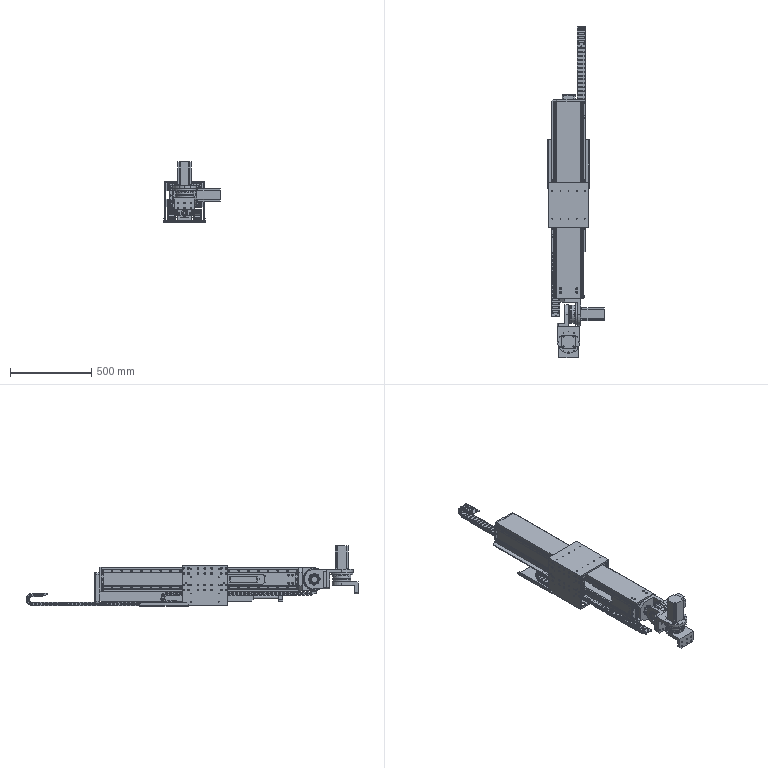Part | SolidWorks | features InContextFeatHolder 23 | 233 solids | 19939 faces | volume 23045702 mm3 | cylinder 9149 | plane 9021 | cone 1529 | torus 92 | spline 76 | sphere 72 | commonest cylinder face diameters 1 x1652 10 x1042 5 x551 20 x487 22 x430 0.2 x408